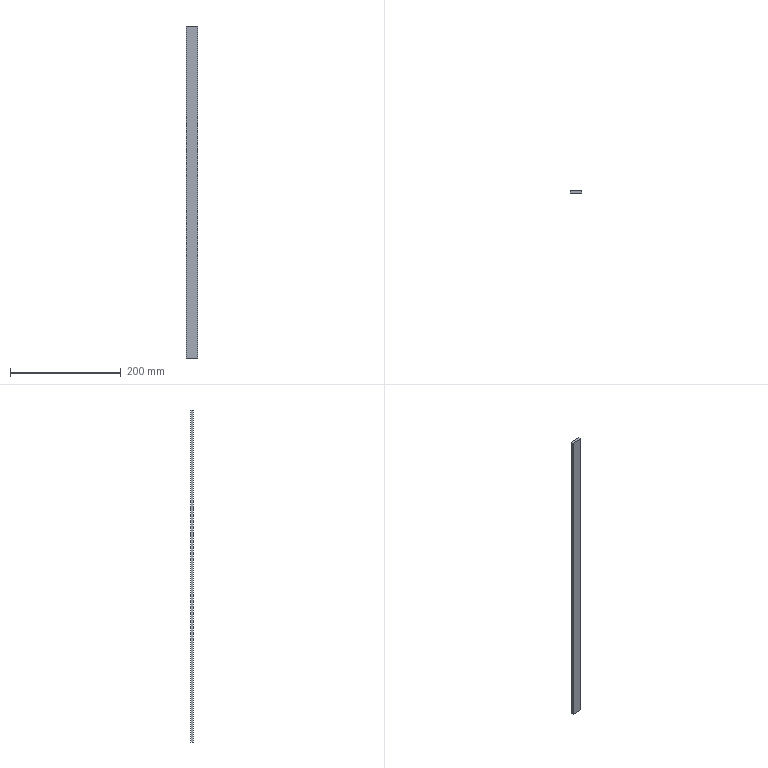Part | STEP file | Guide wheel mechanism revised.sldasm-Part-88 | 1 solid | 6 faces | box 20 x 4.81 x 600 mm | volume 57719 mm3 | plane 6
STEP:
#1=CARTESIAN_POINT('',(130.988,21.64,-600.));
#2=VERTEX_POINT('',#1);
#3=CARTESIAN_POINT('',(130.988,26.45,-600.));
#4=VERTEX_POINT('',#3);
#5=CARTESIAN_POINT('',(130.988,26.45,-600.));
#6=DIRECTION('',(0.,1.,0.));
#7=VECTOR('',#6,1000.);
#8=LINE('',#5,#7);
#9=EDGE_CURVE('',#2,#4,#8,.T.);
#10=ORIENTED_EDGE('',*,*,#9,.F.);
#11=CARTESIAN_POINT('',(130.988,21.64,0.));
#12=VERTEX_POINT('',#11);
#13=CARTESIAN_POINT('',(130.988,21.64,-620.57));
#14=DIRECTION('',(0.,0.,1.));
#15=VECTOR('',#14,1000.);
#16=LINE('',#13,#15);
#17=EDGE_CURVE('',#2,#12,#16,.T.);
#18=ORIENTED_EDGE('',*,*,#17,.T.);
#19=CARTESIAN_POINT('',(130.988,26.45,0.));
#20=VERTEX_POINT('',#19);
#21=CARTESIAN_POINT('',(130.988,26.45,0.));
#22=DIRECTION('',(0.,-1.,0.));
#23=VECTOR('',#22,1000.);
#24=LINE('',#21,#23);
#25=EDGE_CURVE('',#20,#12,#24,.T.);
#26=ORIENTED_EDGE('',*,*,#25,.F.);
#27=CARTESIAN_POINT('',(130.988,26.45,-620.57));
#28=DIRECTION('',(0.,0.,1.));
#29=VECTOR('',#28,1000.);
#30=LINE('',#27,#29);
#31=EDGE_CURVE('',#4,#20,#30,.T.);
#32=ORIENTED_EDGE('',*,*,#31,.F.);
#33=EDGE_LOOP('',(#10,#18,#26,#32));
#34=FACE_OUTER_BOUND('',#33,.T.);
#35=CARTESIAN_POINT('',(130.988,26.45,-620.57));
#36=DIRECTION('',(-1.,0.,0.));
#37=DIRECTION('',(0.,0.,1.));
#38=AXIS2_PLACEMENT_3D('',#35,#36,#37);
#39=PLANE('',#38);
#40=ADVANCED_FACE('',(#34),#39,.T.);
#41=CARTESIAN_POINT('',(150.988,26.45,-600.));
#42=VERTEX_POINT('',#41);
#43=CARTESIAN_POINT('',(130.988,26.45,-600.));
#44=DIRECTION('',(1.,0.,0.));
#45=VECTOR('',#44,1000.);
#46=LINE('',#43,#45);
#47=EDGE_CURVE('',#4,#42,#46,.T.);
#48=ORIENTED_EDGE('',*,*,#47,.F.);
#49=ORIENTED_EDGE('',*,*,#31,.T.);
#50=CARTESIAN_POINT('',(150.988,26.45,0.));
#51=VERTEX_POINT('',#50);
#52=CARTESIAN_POINT('',(130.988,26.45,0.));
#53=DIRECTION('',(-1.,0.,0.));
#54=VECTOR('',#53,1000.);
#55=LINE('',#52,#54);
#56=EDGE_CURVE('',#51,#20,#55,.T.);
#57=ORIENTED_EDGE('',*,*,#56,.F.);
#58=CARTESIAN_POINT('',(150.988,26.45,-620.57));
#59=DIRECTION('',(0.,0.,1.));
#60=VECTOR('',#59,1000.);
#61=LINE('',#58,#60);
#62=EDGE_CURVE('',#42,#51,#61,.T.);
#63=ORIENTED_EDGE('',*,*,#62,.F.);
#64=EDGE_LOOP('',(#48,#49,#57,#63));
#65=FACE_OUTER_BOUND('',#64,.T.);
#66=CARTESIAN_POINT('',(130.988,26.45,-620.57));
#67=DIRECTION('',(0.,1.,0.));
#68=DIRECTION('',(-1.,0.,0.));
#69=AXIS2_PLACEMENT_3D('',#66,#67,#68);
#70=PLANE('',#69);
#71=ADVANCED_FACE('',(#65),#70,.T.);
#72=CARTESIAN_POINT('',(150.988,21.64,-600.));
#73=VERTEX_POINT('',#72);
#74=CARTESIAN_POINT('',(150.988,26.45,-600.));
#75=DIRECTION('',(0.,-1.,0.));
#76=VECTOR('',#75,1000.);
#77=LINE('',#74,#76);
#78=EDGE_CURVE('',#42,#73,#77,.T.);
#79=ORIENTED_EDGE('',*,*,#78,.F.);
#80=ORIENTED_EDGE('',*,*,#62,.T.);
#81=CARTESIAN_POINT('',(150.988,21.64,0.));
#82=VERTEX_POINT('',#81);
#83=CARTESIAN_POINT('',(150.988,26.45,0.));
#84=DIRECTION('',(0.,1.,0.));
#85=VECTOR('',#84,1000.);
#86=LINE('',#83,#85);
#87=EDGE_CURVE('',#82,#51,#86,.T.);
#88=ORIENTED_EDGE('',*,*,#87,.F.);
#89=CARTESIAN_POINT('',(150.988,21.64,-620.57));
#90=DIRECTION('',(0.,0.,1.));
#91=VECTOR('',#90,1000.);
#92=LINE('',#89,#91);
#93=EDGE_CURVE('',#73,#82,#92,.T.);
#94=ORIENTED_EDGE('',*,*,#93,.F.);
#95=EDGE_LOOP('',(#79,#80,#88,#94));
#96=FACE_OUTER_BOUND('',#95,.T.);
#97=CARTESIAN_POINT('',(150.988,26.45,-620.57));
#98=DIRECTION('',(1.,0.,0.));
#99=DIRECTION('',(0.,0.,-1.));
#100=AXIS2_PLACEMENT_3D('',#97,#98,#99);
#101=PLANE('',#100);
#102=ADVANCED_FACE('',(#96),#101,.T.);
#103=CARTESIAN_POINT('',(130.988,21.64,-600.));
#104=DIRECTION('',(-1.,0.,0.));
#105=VECTOR('',#104,1000.);
#106=LINE('',#103,#105);
#107=EDGE_CURVE('',#73,#2,#106,.T.);
#108=ORIENTED_EDGE('',*,*,#107,.F.);
#109=ORIENTED_EDGE('',*,*,#93,.T.);
#110=CARTESIAN_POINT('',(130.988,21.64,0.));
#111=DIRECTION('',(1.,0.,0.));
#112=VECTOR('',#111,1000.);
#113=LINE('',#110,#112);
#114=EDGE_CURVE('',#12,#82,#113,.T.);
#115=ORIENTED_EDGE('',*,*,#114,.F.);
#116=ORIENTED_EDGE('',*,*,#17,.F.);
#117=EDGE_LOOP('',(#108,#109,#115,#116));
#118=FACE_OUTER_BOUND('',#117,.T.);
#119=CARTESIAN_POINT('',(130.988,21.64,-620.57));
#120=DIRECTION('',(0.,-1.,0.));
#121=DIRECTION('',(1.,0.,0.));
#122=AXIS2_PLACEMENT_3D('',#119,#120,#121);
#123=PLANE('',#122);
#124=ADVANCED_FACE('',(#118),#123,.T.);
#125=ORIENTED_EDGE('',*,*,#25,.T.);
#126=ORIENTED_EDGE('',*,*,#114,.T.);
#127=ORIENTED_EDGE('',*,*,#87,.T.);
#128=ORIENTED_EDGE('',*,*,#56,.T.);
#129=EDGE_LOOP('',(#125,#126,#127,#128));
#130=FACE_OUTER_BOUND('',#129,.T.);
#131=CARTESIAN_POINT('',(0.,0.,0.));
#132=DIRECTION('',(0.,0.,1.));
#133=DIRECTION('',(1.,0.,0.));
#134=AXIS2_PLACEMENT_3D('',#131,#132,#133);
#135=PLANE('',#134);
#136=ADVANCED_FACE('',(#130),#135,.T.);
#137=ORIENTED_EDGE('',*,*,#9,.T.);
#138=ORIENTED_EDGE('',*,*,#47,.T.);
#139=ORIENTED_EDGE('',*,*,#78,.T.);
#140=ORIENTED_EDGE('',*,*,#107,.T.);
#141=EDGE_LOOP('',(#137,#138,#139,#140));
#142=FACE_OUTER_BOUND('',#141,.T.);
#143=CARTESIAN_POINT('',(-14.837,-23.55,-600.));
#144=DIRECTION('',(0.,0.,1.));
#145=DIRECTION('',(1.,0.,0.));
#146=AXIS2_PLACEMENT_3D('',#143,#144,#145);
#147=PLANE('',#146);
#148=ADVANCED_FACE('',(#142),#147,.F.);
#149=CLOSED_SHELL('',(#40,#71,#102,#124,#136,#148));
#150=MANIFOLD_SOLID_BREP('',#149);
#151=CARTESIAN_POINT('',(0.,0.,0.));
#152=DIRECTION('',(0.,0.,1.));
#153=DIRECTION('',(1.,0.,0.));
#154=AXIS2_PLACEMENT_3D('',#151,#152,#153);
#155=(LENGTH_UNIT()NAMED_UNIT(*)SI_UNIT(.MILLI.,.METRE.));
#156=UNCERTAINTY_MEASURE_WITH_UNIT(LENGTH_MEASURE(0.00001),#155,'','');
#157=(NAMED_UNIT(*)PLANE_ANGLE_UNIT()SI_UNIT($,.RADIAN.));
#158=(NAMED_UNIT(*)SI_UNIT($,.STERADIAN.)SOLID_ANGLE_UNIT());
#159=(GEOMETRIC_REPRESENTATION_CONTEXT(3)GLOBAL_UNCERTAINTY_ASSIGNED_CONTEXT((#156))GLOBAL_UNIT_ASSIGNED_CONTEXT((#155,#157,#158))REPRESENTATION_CONTEXT('',''));
#160=ADVANCED_BREP_SHAPE_REPRESENTATION('',(#150,#154),#159);